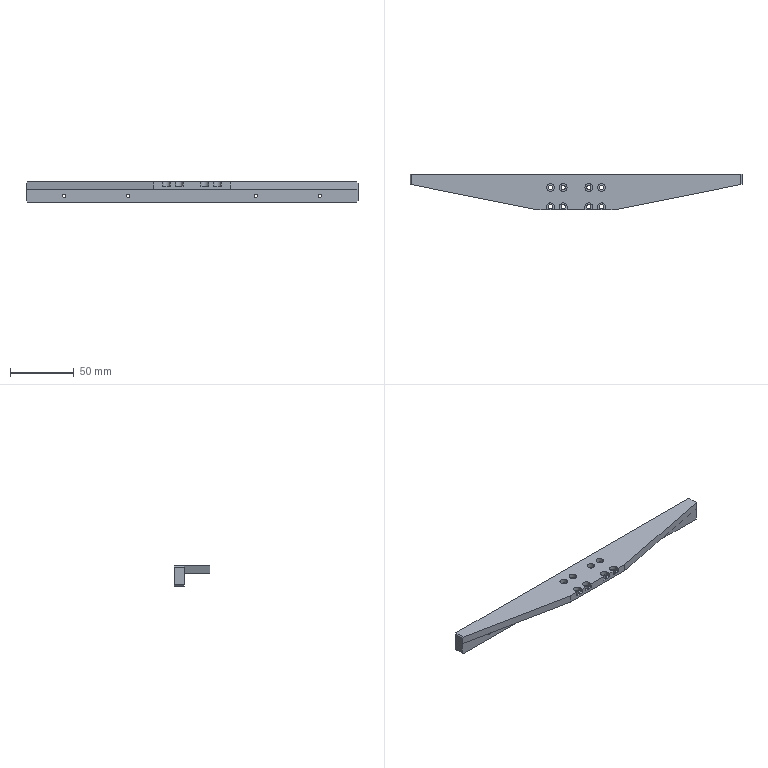NC program | NX | posted with a generic post | part box 260 x 28 x 16 mm
Whole program:
N10 G17 G21 G94 G90
(FLOOR_WALL_COPY , TOOL : D80)
N12 T19 M6
N14 G54
N16 G17 G0 G90 X-173. Y0. B0. C0. S6500 M3
N18 G43 Z30. H19
N20 Z6.
N22 G94 G1 Z3. F1500.
N24 X-170.
N26 X170.
N28 X173.
N30 Z6.
N32 G0 Z30.
N34 X-173.
N36 Z5.
N38 G1 Z2.
N40 X-170.
N42 X170.
N44 X173.
N46 Z5.
N48 G0 Z30.
N50 X-173.
N52 Z4.
N54 G1 Z1.
N56 X-170.
N58 X170.
N60 X173.
N62 Z4.
N64 G0 Z30.
N66 X-173.
N68 Z3.
N70 G1 Z0.
N72 X-170.
N74 X170.
N76 X173.
N78 Z3.
N80 G0 Z30.
N82 M5
(DRILLING , TOOL : D6A45)
N84 T01 M6
N86 G54
N88 G17 G0 G90 X10. Y3.5 B0. C0. S9500 M3
N90 G43 Z30. H1
N92 G94 G81 G98 Z-1. F250. R3.
N94 X20.
N96 Y-11.5
N98 X10.
N100 X-10.
N102 X-20.
N104 Y3.5
N106 X-10.
N108 G80
N110 G0 X-10. Y3.5 Z30.
N112 M5
(DRILLING_COPY , TOOL : 3.4ZT)
N114 T16 M6
N116 G54
N118 G17 G0 G90 X10. Y3.5 B0. C0. S2000 M3
N120 G43 Z30. H16
N122 G94 G83 G98 Z-8.521 F150. Q2. R3.
N124 X20.
N126 Y-11.5
N128 X10.
N130 X-10.
N132 X-20.
N134 Y3.5
N136 X-10.
N138 G80
N140 G0 X-10. Y3.5 Z30.
N142 M5
(HOLE_MILLING , TOOL : D4)
N144 T11 M6
N146 G54
N148 G17 G0 G90 X-20. Y3.5 B0. C0. S9500 M3
N150 G43 Z30. H11
N152 Z0.5
N154 G94 G3 X-19.5 Y3. R0.5 F1250.
N156 X-19. Y3.5 R0.5
N158 X-19. Y3.5 Z0.15 I-1. J0.
N160 X-19. Y3.5 Z-0.2 I-1. J0.
N162 X-19. Y3.5 Z-0.55 I-1. J0.
N164 X-19. Y3.5 Z-0.9 I-1. J0.
N166 X-19. Y3.5 Z-1.25 I-1. J0.
N168 X-19. Y3.5 Z-1.6 I-1. J0.
N170 X-19. Y3.5 Z-1.95 I-1. J0.
N172 X-19. Y3.5 Z-2.3 I-1. J0.
N174 X-19. Y3.5 Z-2.65 I-1. J0.
N176 X-19. Y3.5 Z-3. I-1. J0.
N178 X-19. Y3.5 Z-3.35 I-1. J0.
N180 X-19.377 Y4.282 Z-3.4 R1.
N182 X-20.782 Y4.123 R1.
N184 X-19.377 Y4.282 R-1.
N186 X-20.079 Y4.203 R0.5
N188 X-20. Y3.5 R0.5
N190 G0 Z30.
N192 X-10.
N194 Z0.5
N196 G3 X-9.5 Y3. R0.5
N198 X-9. Y3.5 R0.5
N200 X-9. Y3.5 Z0.15 I-1. J0.
N202 X-9. Y3.5 Z-0.2 I-1. J0.
N204 X-9. Y3.5 Z-0.55 I-1. J0.
N206 X-9. Y3.5 Z-0.9 I-1. J0.
N208 X-9. Y3.5 Z-1.25 I-1. J0.
N210 X-9. Y3.5 Z-1.6 I-1. J0.
N212 X-9. Y3.5 Z-1.95 I-1. J0.
N214 X-9. Y3.5 Z-2.3 I-1. J0.
N216 X-9. Y3.5 Z-2.65 I-1. J0.
N218 X-9. Y3.5 Z-3. I-1. J0.
N220 X-9. Y3.5 Z-3.35 I-1. J0.
N222 X-9.377 Y4.282 Z-3.4 R1.
N224 X-10.782 Y4.123 R1.
N226 X-9.377 Y4.282 R-1.
N228 X-10.079 Y4.203 R0.5
N230 X-10. Y3.5 R0.5
N232 G0 Z30.
N234 X10.
N236 Z0.5
N238 G3 X10.5 Y3. R0.5
N240 X11. Y3.5 R0.5
N242 X11. Y3.5 Z0.15 I-1. J0.
N244 X11. Y3.5 Z-0.2 I-1. J0.
N246 X11. Y3.5 Z-0.55 I-1. J0.
N248 X11. Y3.5 Z-0.9 I-1. J0.
N250 X11. Y3.5 Z-1.25 I-1. J0.
N252 X11. Y3.5 Z-1.6 I-1. J0.
N254 X11. Y3.5 Z-1.95 I-1. J0.
N256 X11. Y3.5 Z-2.3 I-1. J0.
N258 X11. Y3.5 Z-2.65 I-1. J0.
N260 X11. Y3.5 Z-3. I-1. J0.
N262 X11. Y3.5 Z-3.35 I-1. J0.
N264 X10.623 Y4.282 Z-3.4 R1.
N266 X9.218 Y4.123 R1.
N268 X10.623 Y4.282 R-1.
N270 X9.921 Y4.203 R0.5
N272 X10. Y3.5 R0.5
N274 G0 Z30.
N276 X20.
N278 Z0.5
N280 G3 X20.5 Y3. R0.5
N282 X21. Y3.5 R0.5
N284 X21. Y3.5 Z0.15 I-1. J0.
N286 X21. Y3.5 Z-0.2 I-1. J0.
N288 X21. Y3.5 Z-0.55 I-1. J0.
N290 X21. Y3.5 Z-0.9 I-1. J0.
N292 X21. Y3.5 Z-1.25 I-1. J0.
N294 X21. Y3.5 Z-1.6 I-1. J0.
N296 X21. Y3.5 Z-1.95 I-1. J0.
N298 X21. Y3.5 Z-2.3 I-1. J0.
N300 X21. Y3.5 Z-2.65 I-1. J0.
N302 X21. Y3.5 Z-3. I-1. J0.
N304 X21. Y3.5 Z-3.35 I-1. J0.
N306 X20.623 Y4.282 Z-3.4 R1.
N308 X19.218 Y4.123 R1.
N310 X20.623 Y4.282 R-1.
N312 X19.921 Y4.203 R0.5
N314 X20. Y3.5 R0.5
N316 G0 Z30.
(ZLEVEL_PROFILE_1 , TOOL : D4)
N318 X10.628 Y-16.558
N320 Z-0.34
N322 G1 X10.806 Y-16.454 F2000.
N324 G3 X11.003 Y-16.106 R0.4
N326 G1 X11.001 Y-15.827
N328 Y-14.158
N330 X11. Y-14.
N332 Y-11.5
N334 G3 X10. Y-10.5 R1.
N336 X9. Y-11.5 R1.
N338 G1 Y-14.
N340 X8.999 Y-15.827
N342 X8.998 Y-16.106
N344 G3 X9.196 Y-16.453 R0.4
N346 G1 X9.373 Y-16.556
N348 G0 X10.628 Y-16.558 Z-0.68
N350 G1 X10.806 Y-16.454
N352 G3 X11.003 Y-16.106 R0.4
N354 G1 X11.001 Y-15.827
N356 Y-14.158
N358 X11. Y-14.
N360 Y-11.5
N362 G3 X10. Y-10.5 R1.
N364 X9. Y-11.5 R1.
N366 G1 Y-14.
N368 X8.999 Y-15.827
N370 X8.998 Y-16.106
N372 G3 X9.196 Y-16.453 R0.4
N374 G1 X9.373 Y-16.556
N376 G0 X10.628 Y-16.558 Z-1.02
N378 G1 X10.806 Y-16.454
N380 G3 X11.003 Y-16.106 R0.4
N382 G1 X11.001 Y-15.827
N384 Y-14.158
N386 X11. Y-14.
N388 Y-11.5
N390 G3 X10. Y-10.5 R1.
N392 X9. Y-11.5 R1.
N394 G1 Y-14.
N396 Y-15.827
N398 X8.998 Y-16.106
N400 G3 X9.197 Y-16.453 R0.4
N402 G1 X9.373 Y-16.556
N404 G0 X10.628 Y-16.559 Z-1.36
N406 G1 X10.806 Y-16.454
N408 G3 X11.003 Y-16.106 R0.4
N410 G1 X11.001 Y-15.827
N412 X11. Y-14.
N414 Y-11.5
N416 G3 X10. Y-10.5 R1.
N418 X9. Y-11.5 R1.
N420 G1 Y-14.
N422 Y-15.827
N424 X8.998 Y-16.106
N426 G3 X9.197 Y-16.453 R0.4
N428 G1 X9.374 Y-16.556
N430 G0 X10.628 Y-16.559 Z-1.7
N432 G1 X10.806 Y-16.454
N434 G3 X11.003 Y-16.106 R0.4
N436 G1 X11.001 Y-15.827
N438 X11. Y-14.
N440 Y-11.5
N442 G3 X10. Y-10.5 R1.
N444 X9. Y-11.5 R1.
N446 G1 Y-14.
N448 Y-15.827
N450 X8.998 Y-16.106
N452 G3 X9.197 Y-16.453 R0.4
N454 G1 X9.374 Y-16.556
N456 G0 X10.628 Y-16.559 Z-2.04
N458 G1 X10.806 Y-16.454
N460 G3 X11.003 Y-16.106 R0.4
N462 G1 X11. Y-15.827
N464 Y-14.
N466 Y-11.5
N468 G3 X10. Y-10.5 R1.
N470 X9. Y-11.5 R1.
N472 G1 Y-14.
N474 Y-15.827
N476 X8.999 Y-16.106
N478 G3 X9.197 Y-16.453 R0.4
N480 G1 X9.374 Y-16.556
N482 G0 X10.628 Y-16.559 Z-2.38
N484 G1 X10.806 Y-16.454
N486 G3 X11.003 Y-16.106 R0.4
N488 G1 X11. Y-15.827
N490 Y-14.
N492 Y-11.5
N494 G3 X10. Y-10.5 R1.
N496 X9. Y-11.5 R1.
N498 G1 Y-14.
N500 Y-15.827
N502 X8.999 Y-16.106
N504 G3 X9.197 Y-16.453 R0.4
N506 G1 X9.374 Y-16.556
N508 G0 X10.628 Y-16.559 Z-2.72
N510 G1 X10.806 Y-16.454
N512 G3 X11.003 Y-16.106 R0.4
N514 G1 X11. Y-15.827
N516 Y-14.
N518 Y-11.5
N520 G3 X10. Y-10.5 R1.
N522 X9. Y-11.5 R1.
N524 G1 Y-14.
N526 Y-15.827
N528 X8.999 Y-16.106
N530 G3 X9.197 Y-16.453 R0.4
N532 G1 X9.374 Y-16.556
N534 G0 X10.628 Y-16.559 Z-3.06
N536 G1 X10.806 Y-16.454
N538 G3 X11.003 Y-16.106 R0.4
N540 G1 X11. Y-15.827
N542 Y-14.
N544 Y-11.5
N546 G3 X10. Y-10.5 R1.
N548 X9. Y-11.5 R1.
N550 G1 Y-14.
N552 Y-15.827
N554 X8.999 Y-16.106
N556 G3 X9.197 Y-16.453 R0.4
N558 G1 X9.374 Y-16.556
N560 G0 X10.628 Y-16.559 Z-3.4
N562 G1 X10.806 Y-16.454
N564 G3 X11.003 Y-16.106 R0.4
N566 G1 X11. Y-15.827
N568 Y-14.
N570 Y-11.5
N572 G3 X10. Y-10.5 R1.
N574 X9. Y-11.5 R1.
N576 G1 Y-14.
N578 Y-15.827
N580 X8.999 Y-16.106
N582 G3 X9.198 Y-16.453 R0.4
N584 G1 X9.374 Y-16.556
N586 G0 Z30.
N588 X20.627 Y-16.557
N590 Z-0.34
N592 G1 X20.805 Y-16.453
N594 G3 X21.002 Y-16.106 R0.4
N596 G1 X21.001 Y-15.827
N598 X21. Y-14.
N600 Y-11.5
N602 G3 X20. Y-10.5 R1.
N604 X19. Y-11.5 R1.
N606 G1 Y-14.
N608 X18.999 Y-14.158
N610 Y-15.827
N612 X18.997 Y-16.106
N614 G3 X19.195 Y-16.453 R0.4
N616 G1 X19.372 Y-16.557
N618 G0 X20.627 Z-0.68
N620 G1 X20.805 Y-16.453
N622 G3 X21.002 Y-16.106 R0.4
N624 G1 X21.001 Y-15.827
N626 X21. Y-14.
N628 Y-11.5
N630 G3 X20. Y-10.5 R1.
N632 X19. Y-11.5 R1.
N634 G1 Y-14.
N636 X18.999 Y-14.158
N638 Y-15.827
N640 X18.997 Y-16.106
N642 G3 X19.195 Y-16.453 R0.4
N644 G1 X19.372 Y-16.557
N646 G0 X20.627 Z-1.02
N648 G1 X20.805 Y-16.453
N650 G3 X21.002 Y-16.106 R0.4
N652 G1 X21. Y-15.827
N654 Y-14.
N656 Y-11.5
N658 G3 X20. Y-10.5 R1.
N660 X19. Y-11.5 R1.
N662 G1 Y-14.
N664 X18.999 Y-14.158
N666 Y-15.827
N668 X18.998 Y-16.106
N670 G3 X19.196 Y-16.453 R0.4
N672 G1 X19.373 Y-16.557
N674 G0 X20.627 Z-1.36
N676 G1 X20.805 Y-16.453
N678 G3 X21.002 Y-16.106 R0.4
N680 G1 X21. Y-15.827
N682 Y-14.
N684 Y-11.5
N686 G3 X20. Y-10.5 R1.
N688 X19. Y-11.5 R1.
N690 G1 Y-14.
N692 X18.999 Y-15.827
N694 X18.998 Y-16.106
N696 G3 X19.196 Y-16.453 R0.4
N698 G1 X19.373 Y-16.557
N700 G0 X20.627 Z-1.7
N702 G1 X20.805 Y-16.453
N704 G3 X21.002 Y-16.106 R0.4
N706 G1 X21. Y-15.827
N708 Y-14.
N710 Y-11.5
N712 G3 X20. Y-10.5 R1.
N714 X19. Y-11.5 R1.
N716 G1 Y-14.
N718 X18.999 Y-15.827
N720 X18.998 Y-16.106
N722 G3 X19.196 Y-16.453 R0.4
N724 G1 X19.373 Y-16.557
N726 G0 X20.627 Y-16.558 Z-2.04
N728 G1 X20.805 Y-16.453
N730 G3 X21.002 Y-16.106 R0.4
N732 G1 X21. Y-15.827
N734 Y-14.
N736 Y-11.5
N738 G3 X20. Y-10.5 R1.
N740 X19. Y-11.5 R1.
N742 G1 Y-14.
N744 Y-15.827
N746 X18.998 Y-16.106
N748 G3 X19.196 Y-16.453 R0.4
N750 G1 X19.373 Y-16.556
N752 G0 X20.627 Y-16.558 Z-2.38
N754 G1 X20.805 Y-16.453
N756 G3 X21.002 Y-16.106 R0.4
N758 G1 X21. Y-15.827
N760 Y-14.
N762 Y-11.5
N764 G3 X20. Y-10.5 R1.
N766 X19. Y-11.5 R1.
N768 G1 Y-14.
N770 Y-15.827
N772 X18.998 Y-16.106
N774 G3 X19.196 Y-16.453 R0.4
N776 G1 X19.373 Y-16.556
N778 G0 X20.627 Y-16.558 Z-2.72
N780 G1 X20.805 Y-16.453
N782 G3 X21.002 Y-16.106 R0.4
N784 G1 X21. Y-15.827
N786 Y-14.
N788 Y-11.5
N790 G3 X20. Y-10.5 R1.
N792 X19. Y-11.5 R1.
N794 G1 Y-14.
N796 Y-15.827
N798 X18.998 Y-16.106
N800 G3 X19.197 Y-16.453 R0.4
N802 G1 X19.373 Y-16.556
N804 G0 X20.627 Y-16.558 Z-3.06
N806 G1 X20.805 Y-16.454
N808 G3 X21.002 Y-16.106 R0.4
N810 G1 X21. Y-15.827
N812 Y-14.
N814 Y-11.5
N816 G3 X20. Y-10.5 R1.
N818 X19. Y-11.5 R1.
N820 G1 Y-14.
N822 Y-15.827
N824 X18.999 Y-16.106
N826 G3 X19.197 Y-16.453 R0.4
N828 G1 X19.374 Y-16.556
N830 G0 X20.627 Y-16.558 Z-3.4
N832 G1 X20.804 Y-16.454
N834 G3 X21.002 Y-16.106 R0.4
N836 G1 X21. Y-15.827
N838 Y-14.
N840 Y-11.5
N842 G3 X20. Y-10.5 R1.
N844 X19. Y-11.5 R1.
N846 G1 Y-14.
N848 Y-15.827
N850 X18.999 Y-16.106
N852 G3 X19.197 Y-16.453 R0.4
N854 G1 X19.374 Y-16.556
N856 G0 Z30.
N858 X-19.371 Y-16.561
N860 Z-0.34
N862 G1 X-19.192 Y-16.455
N864 G3 X-18.997 Y-16.106 R0.4
N866 G1 X-19. Y-15.827
N868 Y-14.
N870 Y-11.5
N872 G3 X-20. Y-10.5 R1.
N874 X-21. Y-11.5 R1.
N876 G1 Y-14.
N878 X-20.999 Y-14.158
N880 Y-15.827
N882 X-21.002 Y-16.106
N884 G3 X-20.806 Y-16.454 R0.4
N886 G1 X-20.627 Y-16.559
N888 G0 X-19.371 Y-16.561 Z-0.68
N890 G1 X-19.192 Y-16.455
N892 G3 X-18.997 Y-16.106 R0.4
N894 G1 X-19.001 Y-15.827
N896 X-19. Y-14.
N898 Y-11.5
N900 G3 X-20. Y-10.5 R1.
N902 X-21. Y-11.5 R1.
N904 G1 Y-14.
N906 X-20.999 Y-14.158
N908 Y-15.827
N910 X-21.002 Y-16.106
N912 G3 X-20.805 Y-16.454 R0.4
N914 G1 X-20.627 Y-16.559
N916 G0 X-19.371 Y-16.562 Z-1.02
N918 G1 X-19.192 Y-16.455
N920 G3 X-18.997 Y-16.106 R0.4
N922 G1 X-19.001 Y-15.827
N924 X-19. Y-14.
N926 Y-11.5
N928 G3 X-20. Y-10.5 R1.
N930 X-21. Y-11.5 R1.
N932 G1 Y-14.
N934 X-20.999 Y-14.158
N936 Y-15.827
N938 X-21.002 Y-16.106
N940 G3 X-20.805 Y-16.454 R0.4
N942 G1 X-20.627 Y-16.559
N944 G0 X-19.371 Y-16.562 Z-1.36
N946 G1 X-19.192 Y-16.455
N948 G3 X-18.997 Y-16.106 R0.4
N950 G1 X-19.001 Y-15.827
N952 Y-14.158
N954 X-19. Y-14.
N956 Y-11.5
N958 G3 X-20. Y-10.5 R1.
N960 X-21. Y-11.5 R1.
N962 G1 Y-14.
N964 X-20.999 Y-14.158
N966 Y-15.827
N968 X-21.002 Y-16.106
N970 G3 X-20.805 Y-16.454 R0.4
N972 G1 X-20.627 Y-16.559
N974 G0 X-19.371 Y-16.562 Z-1.7
N976 G1 X-19.192 Y-16.455
N978 G3 X-18.997 Y-16.106 R0.4
N980 G1 X-19.001 Y-15.827
N982 Y-14.158
N984 X-19. Y-14.
N986 Y-11.5
N988 G3 X-20. Y-10.5 R1.
N990 X-21. Y-11.5 R1.
N992 G1 Y-14.
N994 X-20.999 Y-14.158
N996 Y-15.827
N998 X-21.002 Y-16.106
N1000 G3 X-20.805 Y-16.454 R0.4
N1002 G1 X-20.627 Y-16.559
N1004 G0 X-19.371 Y-16.562 Z-2.04
N1006 G1 X-19.192 Y-16.455
N1008 G3 X-18.997 Y-16.106 R0.4
N1010 G1 X-19.001 Y-15.827
N1012 Y-14.158
N1014 X-19. Y-14.
N1016 Y-11.5
N1018 G3 X-20. Y-10.5 R1.
N1020 X-21. Y-11.5 R1.
N1022 G1 Y-14.
N1024 X-20.999 Y-14.158
N1026 Y-15.827
N1028 X-21.001 Y-16.106
N1030 G3 X-20.805 Y-16.454 R0.4
N1032 G1 X-20.627 Y-16.559
N1034 G0 X-19.371 Y-16.562 Z-2.38
N1036 G1 X-19.192 Y-16.455
N1038 G3 X-18.997 Y-16.106 R0.4
N1040 G1 X-19.001 Y-15.827
N1042 Y-14.158
N1044 X-19. Y-14.
N1046 Y-11.5
N1048 G3 X-20. Y-10.5 R1.
N1050 X-21. Y-11.5 R1.
N1052 G1 Y-14.
N1054 X-20.998 Y-14.158
N1056 Y-15.827
N1058 X-21.001 Y-16.106
N1060 G3 X-20.805 Y-16.454 R0.4
N1062 G1 X-20.627 Y-16.559
N1064 G0 X-19.371 Y-16.562 Z-2.72
N1066 G1 X-19.192 Y-16.455
N1068 G3 X-18.997 Y-16.106 R0.4
N1070 G1 X-19.001 Y-15.827
N1072 Y-14.158
N1074 X-19. Y-14.
N1076 Y-11.5
N1078 G3 X-20. Y-10.5 R1.
N1080 X-21. Y-11.5 R1.
N1082 G1 Y-14.
N1084 X-20.998 Y-14.158
N1086 Y-15.827
N1088 X-21.001 Y-16.106
N1090 G3 X-20.805 Y-16.454 R0.4
N1092 G1 X-20.626 Y-16.559
N1094 G0 X-19.372 Y-16.562 Z-3.06
N1096 G1 X-19.192 Y-16.455
N1098 G3 X-18.997 Y-16.106 R0.4
N1100 G1 X-19.001 Y-15.827
N1102 Y-14.158
N1104 X-19. Y-14.
N1106 Y-11.5
N1108 G3 X-20. Y-10.5 R1.
N1110 X-21. Y-11.5 R1.
N1112 G1 Y-14.
N1114 X-20.998 Y-14.158
N1116 Y-15.827
N1118 X-21.001 Y-16.106
N1120 G3 X-20.804 Y-16.454 R0.4
N1122 G1 X-20.626 Y-16.559
N1124 G0 X-19.372 Y-16.562 Z-3.4
N1126 G1 X-19.192 Y-16.455
N1128 G3 X-18.997 Y-16.106 R0.4
N1130 G1 X-19.002 Y-15.827
N1132 Y-14.158
N1134 X-19. Y-14.
N1136 Y-11.5
N1138 G3 X-20. Y-10.5 R1.
N1140 X-21. Y-11.5 R1.
N1142 G1 Y-14.
N1144 X-20.998 Y-14.158
N1146 Y-15.827
N1148 X-21.001 Y-16.106
N1150 G3 X-20.804 Y-16.454 R0.4
N1152 G1 X-20.626 Y-16.559
N1154 G0 Z30.
N1156 X-9.372 Y-16.56
N1158 Z-0.34
N1160 G1 X-9.194 Y-16.454
N1162 G3 X-8.998 Y-16.106 R0.4
N1164 G1 X-9.001 Y-15.827
N1166 Y-14.158
N1168 X-9. Y-14.
N1170 Y-11.5
N1172 G3 X-10. Y-10.5 R1.
N1174 X-11. Y-11.5 R1.
N1176 G1 Y-14.
N1178 Y-15.827
N1180 X-11.003 Y-16.106
N1182 G3 X-10.807 Y-16.454 R0.4
N1184 G1 X-10.628 Y-16.56
N1186 G0 X-9.372 Z-0.68
N1188 G1 X-9.194 Y-16.454
N1190 G3 X-8.998 Y-16.106 R0.4
N1192 G1 X-9.001 Y-15.827
N1194 Y-14.158
N1196 X-9. Y-14.
N1198 Y-11.5
N1200 G3 X-10. Y-10.5 R1.
N1202 X-11. Y-11.5 R1.
N1204 G1 Y-14.
N1206 X-10.999 Y-15.827
N1208 X-11.003 Y-16.106
N1210 G3 X-10.806 Y-16.454 R0.4
N1212 G1 X-10.628 Y-16.56
N1214 G0 X-9.372 Z-1.02
N1216 G1 X-9.194 Y-16.454
N1218 G3 X-8.998 Y-16.106 R0.4
N1220 G1 X-9.001 Y-15.827
N1222 Y-14.158
N1224 X-9. Y-14.
N1226 Y-11.5
N1228 G3 X-10. Y-10.5 R1.
N1230 X-11. Y-11.5 R1.
N1232 G1 Y-14.
N1234 X-10.999 Y-15.827
N1236 X-11.002 Y-16.106
N1238 G3 X-10.806 Y-16.454 R0.4
N1240 G1 X-10.628 Y-16.56
N1242 G0 X-9.372 Z-1.36
N1244 G1 X-9.194 Y-16.454
N1246 G3 X-8.998 Y-16.106 R0.4
N1248 G1 X-9.001 Y-15.827
N1250 Y-14.158
N1252 X-9. Y-14.
N1254 Y-11.5
N1256 G3 X-10. Y-10.5 R1.
N1258 X-11. Y-11.5 R1.
N1260 G1 Y-14.
N1262 X-10.999 Y-14.158
N1264 Y-15.827
N1266 X-11.002 Y-16.106
N1268 G3 X-10.806 Y-16.454 R0.4
N1270 G1 X-10.628 Y-16.56
N1272 G0 X-9.372 Y-16.561 Z-1.7
N1274 G1 X-9.194 Y-16.454
N1276 G3 X-8.998 Y-16.106 R0.4
N1278 G1 X-9.001 Y-15.827
N1280 Y-14.158
N1282 X-9. Y-14.
N1284 Y-11.5
N1286 G3 X-10. Y-10.5 R1.
N1288 X-11. Y-11.5 R1.
N1290 G1 Y-14.
N1292 X-10.999 Y-14.158
N1294 Y-15.827
N1296 X-11.002 Y-16.106
N1298 G3 X-10.806 Y-16.454 R0.4
N1300 G1 X-10.628 Y-16.56
N1302 G0 X-9.372 Y-16.561 Z-2.04
N1304 G1 X-9.194 Y-16.454
N1306 G3 X-8.998 Y-16.106 R0.4
N1308 G1 X-9.001 Y-15.827
N1310 Y-14.158
N1312 X-9. Y-14.
N1314 Y-11.5
N1316 G3 X-10. Y-10.5 R1.
N1318 X-11. Y-11.5 R1.
N1320 G1 Y-14.
N1322 X-10.999 Y-14.158
N1324 Y-15.827
N1326 X-11.002 Y-16.106
N1328 G3 X-10.806 Y-16.454 R0.4
N1330 G1 X-10.627 Y-16.559
N1332 G0 X-9.372 Y-16.561 Z-2.38
N1334 G1 X-9.194 Y-16.454
N1336 G3 X-8.998 Y-16.106 R0.4
N1338 G1 X-9.002 Y-15.827
N1340 Y-14.158
N1342 X-9. Y-14.
N1344 Y-11.5
N1346 G3 X-10. Y-10.5 R1.
N1348 X-11. Y-11.5 R1.
N1350 G1 Y-14.
N1352 X-10.999 Y-14.158
N1354 Y-15.827
N1356 X-11.002 Y-16.106
N1358 G3 X-10.805 Y-16.454 R0.4
N1360 G1 X-10.627 Y-16.559
N1362 G0 X-9.372 Y-16.561 Z-2.72
N1364 G1 X-9.194 Y-16.455
N1366 G3 X-8.998 Y-16.106 R0.4
N1368 G1 X-9.002 Y-15.827
N1370 Y-14.158
N1372 X-9. Y-14.
N1374 Y-11.5
N1376 G3 X-10. Y-10.5 R1.
N1378 X-11. Y-11.5 R1.
N1380 G1 Y-14.
N1382 X-10.999 Y-14.158
N1384 Y-15.827
N1386 X-11.002 Y-16.106
N1388 G3 X-10.805 Y-16.454 R0.4
N1390 G1 X-10.627 Y-16.559
N1392 G0 X-9.373 Y-16.561 Z-3.06
N1394 G1 X-9.194 Y-16.455
N1396 G3 X-8.998 Y-16.106 R0.4
N1398 G1 X-9.002 Y-15.827
N1400 Y-14.158
N1402 X-9. Y-14.
N1404 Y-11.5
N1406 G3 X-10. Y-10.5 R1.
N1408 X-11. Y-11.5 R1.
N1410 G1 Y-14.
N1412 X-10.999 Y-14.158
N1414 Y-15.827
N1416 X-11.001 Y-16.106
N1418 G3 X-10.805 Y-16.454 R0.4
N1420 G1 X-10.627 Y-16.559
N1422 G0 X-9.373 Y-16.561 Z-3.4
N1424 G1 X-9.194 Y-16.455
N1426 G3 X-8.998 Y-16.106 R0.4
N1428 G1 X-9.002 Y-15.827
N1430 Y-14.158
N1432 X-9. Y-14.
N1434 Y-11.5
N1436 G3 X-10. Y-10.5 R1.
N1438 X-11. Y-11.5 R1.
N1440 G1 Y-14.
N1442 X-10.998 Y-14.158
N1444 Y-15.827
N1446 X-11.001 Y-16.106
N1448 G3 X-10.805 Y-16.454 R0.4
N1450 G1 X-10.627 Y-16.559
N1452 G0 Z30.
N1454 M5
(PLANAR_MILL_COPY_1 , TOOL : D6A45)
N1456 T01 M6
N1458 G54
N1460 G17 G0 G90 X20.866 Y5.1 B0. C0. S9500 M3
N1462 G43 Z30. H1
N1464 Z0.5
N1466 G94 G1 Z-1. F1250.
N1468 G3 X20. Y5.6 R1.
N1470 X17.9 Y3.5 R2.1
N1472 X20. Y5.6 R-2.1
N1474 X19.134 Y5.1 R1.
N1476 G1 Z0.5
N1478 G0 Z30.
N1480 X10.866
N1482 Z0.5
N1484 G1 Z-1.
N1486 G3 X10. Y5.6 R1.
N1488 X7.9 Y3.5 R2.1
N1490 X10. Y5.6 R-2.1
N1492 X9.134 Y5.1 R1.
N1494 G1 Z0.5
N1496 G0 Z30.
N1498 X-0.866 Y15.4
N1500 Z0.5
N1502 G1 Z-1.
N1504 G3 X0. Y14.9 R1.
N1506 G1 X130.
N1508 G2 X130.9 Y14. R0.9
N1510 G1 Y6.
N1512 G2 X130.177 Y5.117 R0.9
N1514 G1 X129.177 Y4.917
N1516 X30.177 Y-14.883
N1518 X30. Y-14.9
N1520 X23.
N1522 G2 X22.1 Y-14. R0.9
N1524 G1 Y-11.5
N1526 G3 X20. Y-9.4 R2.1
N1528 X17.9 Y-11.5 R2.1
N1530 G1 Y-14.
N1532 G2 X17. Y-14.9 R0.9
N1534 G1 X13.
N1536 G2 X12.1 Y-14. R0.9
N1538 G1 Y-11.5
N1540 G3 X10. Y-9.4 R2.1
N1542 X7.9 Y-11.5 R2.1
N1544 G1 Y-14.
N1546 G2 X7. Y-14.9 R0.9
N1548 G1 X-7.
N1550 G2 X-7.9 Y-14. R0.9
N1552 G1 Y-11.5
N1554 G3 X-10. Y-9.4 R2.1
N1556 X-12.1 Y-11.5 R2.1
N1558 G1 Y-14.
N1560 G2 X-13. Y-14.9 R0.9
N1562 G1 X-17.
N1564 G2 X-17.9 Y-14. R0.9
N1566 G1 Y-11.5
N1568 G3 X-20. Y-9.4 R2.1
N1570 X-22.1 Y-11.5 R2.1
N1572 G1 Y-14.
N1574 G2 X-23. Y-14.9 R0.9
N1576 G1 X-30.
N1578 X-30.177 Y-14.883
N1580 X-129.177 Y4.917
N1582 X-130.177 Y5.117
N1584 G2 X-130.9 Y6. R0.9
N1586 G1 Y14.
N1588 G2 X-130. Y14.9 R0.9
N1590 G1 X0.
N1592 G3 X0.866 Y15.4 R1.
N1594 G1 Z0.5
N1596 G0 Z30.
N1598 X-9.134 Y5.1
N1600 Z0.5
N1602 G1 Z-1.
N1604 G3 X-10. Y5.6 R1.
N1606 X-12.1 Y3.5 R2.1
N1608 X-10. Y5.6 R-2.1
N1610 X-10.866 Y5.1 R1.
N1612 G1 Z0.5
N1614 G0 Z30.
N1616 X-19.134
N1618 Z0.5
N1620 G1 Z-1.
N1622 G3 X-20. Y5.6 R1.
N1624 X-22.1 Y3.5 R2.1
N1626 X-20. Y5.6 R-2.1
N1628 X-20.866 Y5.1 R1.
N1630 G1 Z0.5
N1632 G0 Z30.
N1634 M5
N1636 M2